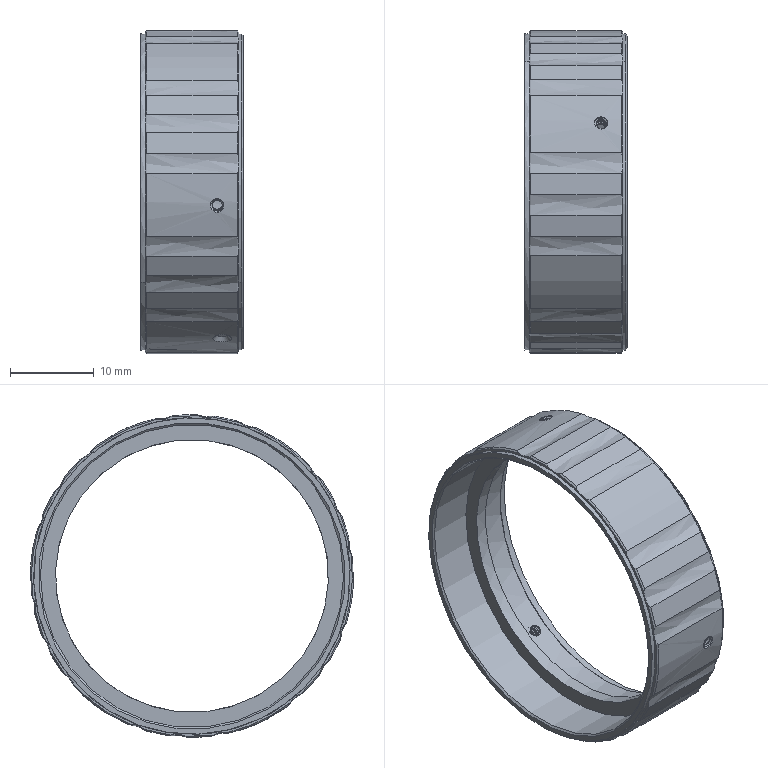Part | SolidWorks | features BaseBody 1 | 1 solid | 173 faces | box 12.2 x 38.6 x 38.6 mm | volume 2092 mm3 | spline 173